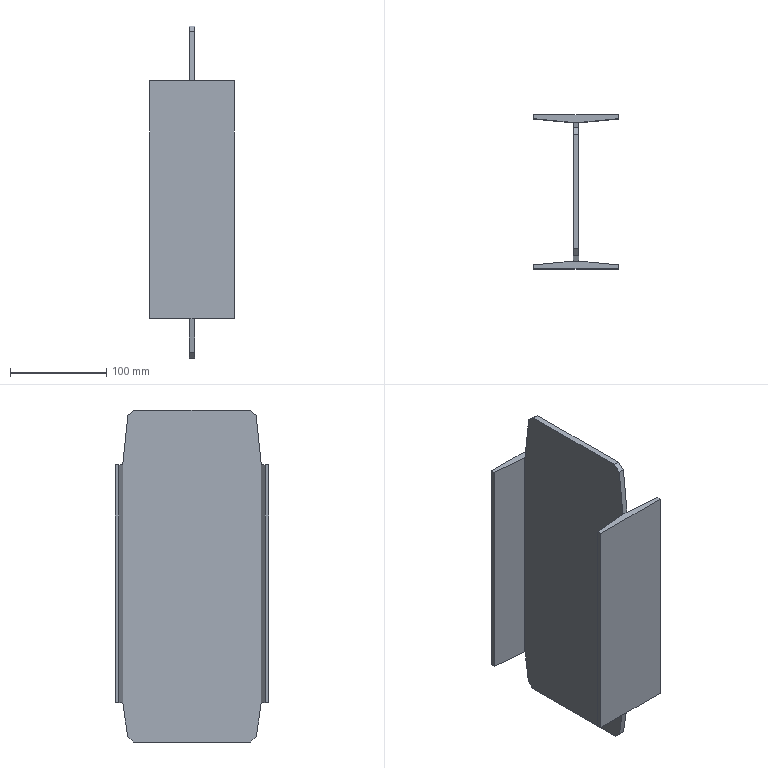Part | SolidWorks | features Chamfer 2, Extrusion 1, ICE 1 | 1 solid | 26 faces | box 88 x 160 x 345 mm | volume 560895 mm3 | plane 26
STEP:
#1=CARTESIAN_POINT('',(44.,-80.,115.5));
#2=VERTEX_POINT('',#1);
#3=CARTESIAN_POINT('',(44.,-80.,-131.5));
#4=VERTEX_POINT('',#3);
#5=CARTESIAN_POINT('',(44.,-80.,172.5));
#6=DIRECTION('',(0.,0.,-1.));
#7=VECTOR('',#6,1000.);
#8=LINE('',#5,#7);
#9=EDGE_CURVE('',#2,#4,#8,.T.);
#10=ORIENTED_EDGE('',*,*,#9,.F.);
#11=CARTESIAN_POINT('',(-44.,-80.,115.5));
#12=VERTEX_POINT('',#11);
#13=CARTESIAN_POINT('',(-44.,-80.,115.5));
#14=DIRECTION('',(1.,0.,0.));
#15=VECTOR('',#14,1000.);
#16=LINE('',#13,#15);
#17=EDGE_CURVE('',#12,#2,#16,.T.);
#18=ORIENTED_EDGE('',*,*,#17,.F.);
#19=CARTESIAN_POINT('',(-44.,-80.,-131.5));
#20=VERTEX_POINT('',#19);
#21=CARTESIAN_POINT('',(-44.,-80.,172.5));
#22=DIRECTION('',(0.,0.,-1.));
#23=VECTOR('',#22,1000.);
#24=LINE('',#21,#23);
#25=EDGE_CURVE('',#12,#20,#24,.T.);
#26=ORIENTED_EDGE('',*,*,#25,.T.);
#27=CARTESIAN_POINT('',(-44.,-80.,-131.5));
#28=DIRECTION('',(1.,0.,0.));
#29=VECTOR('',#28,1000.);
#30=LINE('',#27,#29);
#31=EDGE_CURVE('',#20,#4,#30,.T.);
#32=ORIENTED_EDGE('',*,*,#31,.T.);
#33=EDGE_LOOP('',(#10,#18,#26,#32));
#34=FACE_OUTER_BOUND('',#33,.T.);
#35=CARTESIAN_POINT('',(44.,-80.,172.5));
#36=DIRECTION('',(0.,1.,0.));
#37=DIRECTION('',(-1.,0.,0.));
#38=AXIS2_PLACEMENT_3D('',#35,#36,#37);
#39=PLANE('',#38);
#40=ADVANCED_FACE('',(#34),#39,.F.);
#41=CARTESIAN_POINT('',(44.,-76.,115.5));
#42=VERTEX_POINT('',#41);
#43=CARTESIAN_POINT('',(44.,-76.,-131.5));
#44=VERTEX_POINT('',#43);
#45=CARTESIAN_POINT('',(44.,-76.,172.5));
#46=DIRECTION('',(0.,0.,-1.));
#47=VECTOR('',#46,1000.);
#48=LINE('',#45,#47);
#49=EDGE_CURVE('',#42,#44,#48,.T.);
#50=ORIENTED_EDGE('',*,*,#49,.F.);
#51=CARTESIAN_POINT('',(44.,-72.,115.5));
#52=DIRECTION('',(0.,1.,0.));
#53=VECTOR('',#52,1000.);
#54=LINE('',#51,#53);
#55=EDGE_CURVE('',#2,#42,#54,.T.);
#56=ORIENTED_EDGE('',*,*,#55,.F.);
#57=ORIENTED_EDGE('',*,*,#9,.T.);
#58=CARTESIAN_POINT('',(44.,-72.,-131.5));
#59=DIRECTION('',(0.,-1.,0.));
#60=VECTOR('',#59,1000.);
#61=LINE('',#58,#60);
#62=EDGE_CURVE('',#44,#4,#61,.T.);
#63=ORIENTED_EDGE('',*,*,#62,.F.);
#64=EDGE_LOOP('',(#50,#56,#57,#63));
#65=FACE_OUTER_BOUND('',#64,.T.);
#66=CARTESIAN_POINT('',(44.,-80.,172.5));
#67=DIRECTION('',(-1.,0.,0.));
#68=DIRECTION('',(0.,-1.,0.));
#69=AXIS2_PLACEMENT_3D('',#66,#67,#68);
#70=PLANE('',#69);
#71=ADVANCED_FACE('',(#65),#70,.F.);
#72=CARTESIAN_POINT('',(3.,-72.,115.5));
#73=VERTEX_POINT('',#72);
#74=CARTESIAN_POINT('',(3.,-72.,-131.5));
#75=VERTEX_POINT('',#74);
#76=CARTESIAN_POINT('',(3.,-72.,172.5));
#77=DIRECTION('',(0.,0.,-1.));
#78=VECTOR('',#77,1000.);
#79=LINE('',#76,#78);
#80=EDGE_CURVE('',#73,#75,#79,.T.);
#81=ORIENTED_EDGE('',*,*,#80,.F.);
#82=CARTESIAN_POINT('',(44.,-76.,115.5));
#83=DIRECTION('',(0.9953,-0.0971,0.));
#84=VECTOR('',#83,1000.);
#85=LINE('',#82,#84);
#86=EDGE_CURVE('',#73,#42,#85,.T.);
#87=ORIENTED_EDGE('',*,*,#86,.T.);
#88=ORIENTED_EDGE('',*,*,#49,.T.);
#89=CARTESIAN_POINT('',(44.,-76.,-131.5));
#90=DIRECTION('',(-0.9953,0.0971,0.));
#91=VECTOR('',#90,1000.);
#92=LINE('',#89,#91);
#93=EDGE_CURVE('',#44,#75,#92,.T.);
#94=ORIENTED_EDGE('',*,*,#93,.T.);
#95=EDGE_LOOP('',(#81,#87,#88,#94));
#96=FACE_OUTER_BOUND('',#95,.T.);
#97=CARTESIAN_POINT('',(44.,-76.,172.5));
#98=DIRECTION('',(-0.0971,-0.9953,0.));
#99=DIRECTION('',(0.9953,-0.0971,0.));
#100=AXIS2_PLACEMENT_3D('',#97,#98,#99);
#101=PLANE('',#100);
#102=ADVANCED_FACE('',(#96),#101,.F.);
#103=CARTESIAN_POINT('',(3.,-66.857,-166.643));
#104=VERTEX_POINT('',#103);
#105=CARTESIAN_POINT('',(3.,-112.536,145.495));
#106=DIRECTION('',(0.,0.1448,-0.9895));
#107=VECTOR('',#106,1000.);
#108=LINE('',#105,#107);
#109=EDGE_CURVE('',#75,#104,#108,.T.);
#110=ORIENTED_EDGE('',*,*,#109,.T.);
#111=CARTESIAN_POINT('',(3.,-61.,-172.5));
#112=VERTEX_POINT('',#111);
#113=CARTESIAN_POINT('',(3.,-66.857,-166.643));
#114=DIRECTION('',(0.,0.7071,-0.7071));
#115=VECTOR('',#114,1000.);
#116=LINE('',#113,#115);
#117=EDGE_CURVE('',#104,#112,#116,.T.);
#118=ORIENTED_EDGE('',*,*,#117,.T.);
#119=CARTESIAN_POINT('',(3.,61.,-172.5));
#120=VERTEX_POINT('',#119);
#121=CARTESIAN_POINT('',(3.,72.,-172.5));
#122=DIRECTION('',(0.,1.,0.));
#123=VECTOR('',#122,1000.);
#124=LINE('',#121,#123);
#125=EDGE_CURVE('',#112,#120,#124,.T.);
#126=ORIENTED_EDGE('',*,*,#125,.T.);
#127=CARTESIAN_POINT('',(3.,66.857,-166.643));
#128=VERTEX_POINT('',#127);
#129=CARTESIAN_POINT('',(3.,66.857,-166.643));
#130=DIRECTION('',(0.,0.7071,0.7071));
#131=VECTOR('',#130,1000.);
#132=LINE('',#129,#131);
#133=EDGE_CURVE('',#120,#128,#132,.T.);
#134=ORIENTED_EDGE('',*,*,#133,.T.);
#135=CARTESIAN_POINT('',(3.,72.,-131.5));
#136=VERTEX_POINT('',#135);
#137=CARTESIAN_POINT('',(3.,115.555,166.126));
#138=DIRECTION('',(0.,0.1448,0.9895));
#139=VECTOR('',#138,1000.);
#140=LINE('',#137,#139);
#141=EDGE_CURVE('',#128,#136,#140,.T.);
#142=ORIENTED_EDGE('',*,*,#141,.T.);
#143=CARTESIAN_POINT('',(3.,72.,115.5));
#144=VERTEX_POINT('',#143);
#145=CARTESIAN_POINT('',(3.,72.,172.5));
#146=DIRECTION('',(0.,0.,-1.));
#147=VECTOR('',#146,1000.);
#148=LINE('',#145,#147);
#149=EDGE_CURVE('',#144,#136,#148,.T.);
#150=ORIENTED_EDGE('',*,*,#149,.F.);
#151=CARTESIAN_POINT('',(3.,66.628,166.533));
#152=VERTEX_POINT('',#151);
#153=CARTESIAN_POINT('',(3.,66.066,171.875));
#154=DIRECTION('',(0.,-0.1047,0.9945));
#155=VECTOR('',#154,1000.);
#156=LINE('',#153,#155);
#157=EDGE_CURVE('',#144,#152,#156,.T.);
#158=ORIENTED_EDGE('',*,*,#157,.T.);
#159=CARTESIAN_POINT('',(3.,59.257,172.5));
#160=VERTEX_POINT('',#159);
#161=CARTESIAN_POINT('',(3.,59.257,172.5));
#162=DIRECTION('',(0.,-0.7772,0.6292));
#163=VECTOR('',#162,1000.);
#164=LINE('',#161,#163);
#165=EDGE_CURVE('',#152,#160,#164,.T.);
#166=ORIENTED_EDGE('',*,*,#165,.T.);
#167=CARTESIAN_POINT('',(3.,-59.257,172.5));
#168=VERTEX_POINT('',#167);
#169=CARTESIAN_POINT('',(3.,72.,172.5));
#170=DIRECTION('',(0.,1.,0.));
#171=VECTOR('',#170,1000.);
#172=LINE('',#169,#171);
#173=EDGE_CURVE('',#168,#160,#172,.T.);
#174=ORIENTED_EDGE('',*,*,#173,.F.);
#175=CARTESIAN_POINT('',(3.,-66.628,166.533));
#176=VERTEX_POINT('',#175);
#177=CARTESIAN_POINT('',(3.,-59.257,172.5));
#178=DIRECTION('',(0.,-0.7772,-0.6292));
#179=VECTOR('',#178,1000.);
#180=LINE('',#177,#179);
#181=EDGE_CURVE('',#168,#176,#180,.T.);
#182=ORIENTED_EDGE('',*,*,#181,.T.);
#183=CARTESIAN_POINT('',(3.,-64.488,186.867));
#184=DIRECTION('',(0.,-0.1047,-0.9945));
#185=VECTOR('',#184,1000.);
#186=LINE('',#183,#185);
#187=EDGE_CURVE('',#176,#73,#186,.T.);
#188=ORIENTED_EDGE('',*,*,#187,.T.);
#189=ORIENTED_EDGE('',*,*,#80,.T.);
#190=EDGE_LOOP('',(#110,#118,#126,#134,#142,#150,#158,#166,#174,#182,#188,#189));
#191=FACE_OUTER_BOUND('',#190,.T.);
#192=CARTESIAN_POINT('',(3.,72.,172.5));
#193=DIRECTION('',(-1.,0.,0.));
#194=DIRECTION('',(0.,0.,1.));
#195=AXIS2_PLACEMENT_3D('',#192,#193,#194);
#196=PLANE('',#195);
#197=ADVANCED_FACE('',(#191),#196,.F.);
#198=ORIENTED_EDGE('',*,*,#149,.T.);
#199=CARTESIAN_POINT('',(44.,76.,-131.5));
#200=VERTEX_POINT('',#199);
#201=CARTESIAN_POINT('',(44.,76.,-131.5));
#202=DIRECTION('',(0.9953,0.0971,0.));
#203=VECTOR('',#202,1000.);
#204=LINE('',#201,#203);
#205=EDGE_CURVE('',#136,#200,#204,.T.);
#206=ORIENTED_EDGE('',*,*,#205,.T.);
#207=CARTESIAN_POINT('',(44.,76.,115.5));
#208=VERTEX_POINT('',#207);
#209=CARTESIAN_POINT('',(44.,76.,172.5));
#210=DIRECTION('',(0.,0.,-1.));
#211=VECTOR('',#210,1000.);
#212=LINE('',#209,#211);
#213=EDGE_CURVE('',#208,#200,#212,.T.);
#214=ORIENTED_EDGE('',*,*,#213,.F.);
#215=CARTESIAN_POINT('',(44.,76.,115.5));
#216=DIRECTION('',(-0.9953,-0.0971,0.));
#217=VECTOR('',#216,1000.);
#218=LINE('',#215,#217);
#219=EDGE_CURVE('',#208,#144,#218,.T.);
#220=ORIENTED_EDGE('',*,*,#219,.T.);
#221=EDGE_LOOP('',(#198,#206,#214,#220));
#222=FACE_OUTER_BOUND('',#221,.T.);
#223=CARTESIAN_POINT('',(44.,76.,172.5));
#224=DIRECTION('',(-0.0971,0.9953,0.));
#225=DIRECTION('',(-0.9953,-0.0971,0.));
#226=AXIS2_PLACEMENT_3D('',#223,#224,#225);
#227=PLANE('',#226);
#228=ADVANCED_FACE('',(#222),#227,.F.);
#229=ORIENTED_EDGE('',*,*,#213,.T.);
#230=CARTESIAN_POINT('',(44.,80.,-131.5));
#231=VERTEX_POINT('',#230);
#232=CARTESIAN_POINT('',(44.,72.,-131.5));
#233=DIRECTION('',(0.,-1.,0.));
#234=VECTOR('',#233,1000.);
#235=LINE('',#232,#234);
#236=EDGE_CURVE('',#231,#200,#235,.T.);
#237=ORIENTED_EDGE('',*,*,#236,.F.);
#238=CARTESIAN_POINT('',(44.,80.,115.5));
#239=VERTEX_POINT('',#238);
#240=CARTESIAN_POINT('',(44.,80.,172.5));
#241=DIRECTION('',(0.,0.,-1.));
#242=VECTOR('',#241,1000.);
#243=LINE('',#240,#242);
#244=EDGE_CURVE('',#239,#231,#243,.T.);
#245=ORIENTED_EDGE('',*,*,#244,.F.);
#246=CARTESIAN_POINT('',(44.,72.,115.5));
#247=DIRECTION('',(0.,1.,0.));
#248=VECTOR('',#247,1000.);
#249=LINE('',#246,#248);
#250=EDGE_CURVE('',#208,#239,#249,.T.);
#251=ORIENTED_EDGE('',*,*,#250,.F.);
#252=EDGE_LOOP('',(#229,#237,#245,#251));
#253=FACE_OUTER_BOUND('',#252,.T.);
#254=CARTESIAN_POINT('',(44.,80.,172.5));
#255=DIRECTION('',(-1.,0.,0.));
#256=DIRECTION('',(0.,0.,1.));
#257=AXIS2_PLACEMENT_3D('',#254,#255,#256);
#258=PLANE('',#257);
#259=ADVANCED_FACE('',(#253),#258,.F.);
#260=ORIENTED_EDGE('',*,*,#244,.T.);
#261=CARTESIAN_POINT('',(-44.,80.,-131.5));
#262=VERTEX_POINT('',#261);
#263=CARTESIAN_POINT('',(-44.,80.,-131.5));
#264=DIRECTION('',(1.,0.,0.));
#265=VECTOR('',#264,1000.);
#266=LINE('',#263,#265);
#267=EDGE_CURVE('',#262,#231,#266,.T.);
#268=ORIENTED_EDGE('',*,*,#267,.F.);
#269=CARTESIAN_POINT('',(-44.,80.,115.5));
#270=VERTEX_POINT('',#269);
#271=CARTESIAN_POINT('',(-44.,80.,172.5));
#272=DIRECTION('',(0.,0.,-1.));
#273=VECTOR('',#272,1000.);
#274=LINE('',#271,#273);
#275=EDGE_CURVE('',#270,#262,#274,.T.);
#276=ORIENTED_EDGE('',*,*,#275,.F.);
#277=CARTESIAN_POINT('',(-44.,80.,115.5));
#278=DIRECTION('',(1.,0.,0.));
#279=VECTOR('',#278,1000.);
#280=LINE('',#277,#279);
#281=EDGE_CURVE('',#270,#239,#280,.T.);
#282=ORIENTED_EDGE('',*,*,#281,.T.);
#283=EDGE_LOOP('',(#260,#268,#276,#282));
#284=FACE_OUTER_BOUND('',#283,.T.);
#285=CARTESIAN_POINT('',(44.,80.,172.5));
#286=DIRECTION('',(0.,-1.,0.));
#287=DIRECTION('',(1.,0.,0.));
#288=AXIS2_PLACEMENT_3D('',#285,#286,#287);
#289=PLANE('',#288);
#290=ADVANCED_FACE('',(#284),#289,.F.);
#291=ORIENTED_EDGE('',*,*,#275,.T.);
#292=CARTESIAN_POINT('',(-44.,76.,-131.5));
#293=VERTEX_POINT('',#292);
#294=CARTESIAN_POINT('',(-44.,72.,-131.5));
#295=DIRECTION('',(0.,-1.,0.));
#296=VECTOR('',#295,1000.);
#297=LINE('',#294,#296);
#298=EDGE_CURVE('',#262,#293,#297,.T.);
#299=ORIENTED_EDGE('',*,*,#298,.T.);
#300=CARTESIAN_POINT('',(-44.,76.,115.5));
#301=VERTEX_POINT('',#300);
#302=CARTESIAN_POINT('',(-44.,76.,172.5));
#303=DIRECTION('',(0.,0.,-1.));
#304=VECTOR('',#303,1000.);
#305=LINE('',#302,#304);
#306=EDGE_CURVE('',#301,#293,#305,.T.);
#307=ORIENTED_EDGE('',*,*,#306,.F.);
#308=CARTESIAN_POINT('',(-44.,72.,115.5));
#309=DIRECTION('',(0.,1.,0.));
#310=VECTOR('',#309,1000.);
#311=LINE('',#308,#310);
#312=EDGE_CURVE('',#301,#270,#311,.T.);
#313=ORIENTED_EDGE('',*,*,#312,.T.);
#314=EDGE_LOOP('',(#291,#299,#307,#313));
#315=FACE_OUTER_BOUND('',#314,.T.);
#316=CARTESIAN_POINT('',(-44.,80.,172.5));
#317=DIRECTION('',(1.,0.,0.));
#318=DIRECTION('',(0.,1.,0.));
#319=AXIS2_PLACEMENT_3D('',#316,#317,#318);
#320=PLANE('',#319);
#321=ADVANCED_FACE('',(#315),#320,.F.);
#322=ORIENTED_EDGE('',*,*,#306,.T.);
#323=CARTESIAN_POINT('',(-3.,72.,-131.5));
#324=VERTEX_POINT('',#323);
#325=CARTESIAN_POINT('',(-44.,76.,-131.5));
#326=DIRECTION('',(0.9953,-0.0971,0.));
#327=VECTOR('',#326,1000.);
#328=LINE('',#325,#327);
#329=EDGE_CURVE('',#293,#324,#328,.T.);
#330=ORIENTED_EDGE('',*,*,#329,.T.);
#331=CARTESIAN_POINT('',(-3.,72.,115.5));
#332=VERTEX_POINT('',#331);
#333=CARTESIAN_POINT('',(-3.,72.,172.5));
#334=DIRECTION('',(0.,0.,-1.));
#335=VECTOR('',#334,1000.);
#336=LINE('',#333,#335);
#337=EDGE_CURVE('',#332,#324,#336,.T.);
#338=ORIENTED_EDGE('',*,*,#337,.F.);
#339=CARTESIAN_POINT('',(-44.,76.,115.5));
#340=DIRECTION('',(-0.9953,0.0971,0.));
#341=VECTOR('',#340,1000.);
#342=LINE('',#339,#341);
#343=EDGE_CURVE('',#332,#301,#342,.T.);
#344=ORIENTED_EDGE('',*,*,#343,.T.);
#345=EDGE_LOOP('',(#322,#330,#338,#344));
#346=FACE_OUTER_BOUND('',#345,.T.);
#347=CARTESIAN_POINT('',(-44.,76.,172.5));
#348=DIRECTION('',(0.0971,0.9953,0.));
#349=DIRECTION('',(-0.9953,0.0971,0.));
#350=AXIS2_PLACEMENT_3D('',#347,#348,#349);
#351=PLANE('',#350);
#352=ADVANCED_FACE('',(#346),#351,.F.);
#353=CARTESIAN_POINT('',(-3.,61.,-172.5));
#354=VERTEX_POINT('',#353);
#355=CARTESIAN_POINT('',(-3.,-61.,-172.5));
#356=VERTEX_POINT('',#355);
#357=CARTESIAN_POINT('',(-3.,72.,-172.5));
#358=DIRECTION('',(0.,-1.,0.));
#359=VECTOR('',#358,1000.);
#360=LINE('',#357,#359);
#361=EDGE_CURVE('',#354,#356,#360,.T.);
#362=ORIENTED_EDGE('',*,*,#361,.T.);
#363=CARTESIAN_POINT('',(-3.,-66.857,-166.643));
#364=VERTEX_POINT('',#363);
#365=CARTESIAN_POINT('',(-3.,-66.857,-166.643));
#366=DIRECTION('',(0.,-0.7071,0.7071));
#367=VECTOR('',#366,1000.);
#368=LINE('',#365,#367);
#369=EDGE_CURVE('',#356,#364,#368,.T.);
#370=ORIENTED_EDGE('',*,*,#369,.T.);
#371=CARTESIAN_POINT('',(-3.,-72.,-131.5));
#372=VERTEX_POINT('',#371);
#373=CARTESIAN_POINT('',(-3.,-112.536,145.495));
#374=DIRECTION('',(0.,-0.1448,0.9895));
#375=VECTOR('',#374,1000.);
#376=LINE('',#373,#375);
#377=EDGE_CURVE('',#364,#372,#376,.T.);
#378=ORIENTED_EDGE('',*,*,#377,.T.);
#379=CARTESIAN_POINT('',(-3.,-72.,115.5));
#380=VERTEX_POINT('',#379);
#381=CARTESIAN_POINT('',(-3.,-72.,172.5));
#382=DIRECTION('',(0.,0.,-1.));
#383=VECTOR('',#382,1000.);
#384=LINE('',#381,#383);
#385=EDGE_CURVE('',#380,#372,#384,.T.);
#386=ORIENTED_EDGE('',*,*,#385,.F.);
#387=CARTESIAN_POINT('',(-3.,-66.628,166.533));
#388=VERTEX_POINT('',#387);
#389=CARTESIAN_POINT('',(-3.,-64.488,186.867));
#390=DIRECTION('',(0.,0.1047,0.9945));
#391=VECTOR('',#390,1000.);
#392=LINE('',#389,#391);
#393=EDGE_CURVE('',#380,#388,#392,.T.);
#394=ORIENTED_EDGE('',*,*,#393,.T.);
#395=CARTESIAN_POINT('',(-3.,-59.257,172.5));
#396=VERTEX_POINT('',#395);
#397=CARTESIAN_POINT('',(-3.,-59.257,172.5));
#398=DIRECTION('',(0.,0.7772,0.6292));
#399=VECTOR('',#398,1000.);
#400=LINE('',#397,#399);
#401=EDGE_CURVE('',#388,#396,#400,.T.);
#402=ORIENTED_EDGE('',*,*,#401,.T.);
#403=CARTESIAN_POINT('',(-3.,59.257,172.5));
#404=VERTEX_POINT('',#403);
#405=CARTESIAN_POINT('',(-3.,72.,172.5));
#406=DIRECTION('',(0.,-1.,0.));
#407=VECTOR('',#406,1000.);
#408=LINE('',#405,#407);
#409=EDGE_CURVE('',#404,#396,#408,.T.);
#410=ORIENTED_EDGE('',*,*,#409,.F.);
#411=CARTESIAN_POINT('',(-3.,66.628,166.533));
#412=VERTEX_POINT('',#411);
#413=CARTESIAN_POINT('',(-3.,59.257,172.5));
#414=DIRECTION('',(0.,0.7772,-0.6292));
#415=VECTOR('',#414,1000.);
#416=LINE('',#413,#415);
#417=EDGE_CURVE('',#404,#412,#416,.T.);
#418=ORIENTED_EDGE('',*,*,#417,.T.);
#419=CARTESIAN_POINT('',(-3.,66.066,171.875));
#420=DIRECTION('',(0.,0.1047,-0.9945));
#421=VECTOR('',#420,1000.);
#422=LINE('',#419,#421);
#423=EDGE_CURVE('',#412,#332,#422,.T.);
#424=ORIENTED_EDGE('',*,*,#423,.T.);
#425=ORIENTED_EDGE('',*,*,#337,.T.);
#426=CARTESIAN_POINT('',(-3.,66.857,-166.643));
#427=VERTEX_POINT('',#426);
#428=CARTESIAN_POINT('',(-3.,115.555,166.126));
#429=DIRECTION('',(0.,-0.1448,-0.9895));
#430=VECTOR('',#429,1000.);
#431=LINE('',#428,#430);
#432=EDGE_CURVE('',#324,#427,#431,.T.);
#433=ORIENTED_EDGE('',*,*,#432,.T.);
#434=CARTESIAN_POINT('',(-3.,66.857,-166.643));
#435=DIRECTION('',(0.,-0.7071,-0.7071));
#436=VECTOR('',#435,1000.);
#437=LINE('',#434,#436);
#438=EDGE_CURVE('',#427,#354,#437,.T.);
#439=ORIENTED_EDGE('',*,*,#438,.T.);
#440=EDGE_LOOP('',(#362,#370,#378,#386,#394,#402,#410,#418,#424,#425,#433,#439));
#441=FACE_OUTER_BOUND('',#440,.T.);
#442=CARTESIAN_POINT('',(-3.,72.,172.5));
#443=DIRECTION('',(1.,0.,0.));
#444=DIRECTION('',(0.,0.,-1.));
#445=AXIS2_PLACEMENT_3D('',#442,#443,#444);
#446=PLANE('',#445);
#447=ADVANCED_FACE('',(#441),#446,.F.);
#448=CARTESIAN_POINT('',(-44.,-76.,115.5));
#449=VERTEX_POINT('',#448);
#450=CARTESIAN_POINT('',(-44.,-76.,-131.5));
#451=VERTEX_POINT('',#450);
#452=CARTESIAN_POINT('',(-44.,-76.,172.5));
#453=DIRECTION('',(0.,0.,-1.));
#454=VECTOR('',#453,1000.);
#455=LINE('',#452,#454);
#456=EDGE_CURVE('',#449,#451,#455,.T.);
#457=ORIENTED_EDGE('',*,*,#456,.F.);
#458=CARTESIAN_POINT('',(-44.,-76.,115.5));
#459=DIRECTION('',(0.9953,0.0971,0.));
#460=VECTOR('',#459,1000.);
#461=LINE('',#458,#460);
#462=EDGE_CURVE('',#449,#380,#461,.T.);
#463=ORIENTED_EDGE('',*,*,#462,.T.);
#464=ORIENTED_EDGE('',*,*,#385,.T.);
#465=CARTESIAN_POINT('',(-44.,-76.,-131.5));
#466=DIRECTION('',(-0.9953,-0.0971,0.));
#467=VECTOR('',#466,1000.);
#468=LINE('',#465,#467);
#469=EDGE_CURVE('',#372,#451,#468,.T.);
#470=ORIENTED_EDGE('',*,*,#469,.T.);
#471=EDGE_LOOP('',(#457,#463,#464,#470));
#472=FACE_OUTER_BOUND('',#471,.T.);
#473=CARTESIAN_POINT('',(-44.,-76.,172.5));
#474=DIRECTION('',(0.0971,-0.9953,0.));
#475=DIRECTION('',(0.9953,0.0971,0.));
#476=AXIS2_PLACEMENT_3D('',#473,#474,#475);
#477=PLANE('',#476);
#478=ADVANCED_FACE('',(#472),#477,.F.);
#479=ORIENTED_EDGE('',*,*,#25,.F.);
#480=CARTESIAN_POINT('',(-44.,-72.,115.5));
#481=DIRECTION('',(0.,1.,0.));
#482=VECTOR('',#481,1000.);
#483=LINE('',#480,#482);
#484=EDGE_CURVE('',#12,#449,#483,.T.);
#485=ORIENTED_EDGE('',*,*,#484,.T.);
#486=ORIENTED_EDGE('',*,*,#456,.T.);
#487=CARTESIAN_POINT('',(-44.,-72.,-131.5));
#488=DIRECTION('',(0.,-1.,0.));
#489=VECTOR('',#488,1000.);
#490=LINE('',#487,#489);
#491=EDGE_CURVE('',#451,#20,#490,.T.);
#492=ORIENTED_EDGE('',*,*,#491,.T.);
#493=EDGE_LOOP('',(#479,#485,#486,#492));
#494=FACE_OUTER_BOUND('',#493,.T.);
#495=CARTESIAN_POINT('',(-44.,-80.,172.5));
#496=DIRECTION('',(1.,0.,0.));
#497=DIRECTION('',(0.,1.,0.));
#498=AXIS2_PLACEMENT_3D('',#495,#496,#497);
#499=PLANE('',#498);
#500=ADVANCED_FACE('',(#494),#499,.F.);
#501=ORIENTED_EDGE('',*,*,#409,.T.);
#502=CARTESIAN_POINT('',(0.,-59.257,172.5));
#503=DIRECTION('',(1.,0.,0.));
#504=VECTOR('',#503,1000.);
#505=LINE('',#502,#504);
#506=EDGE_CURVE('',#396,#168,#505,.T.);
#507=ORIENTED_EDGE('',*,*,#506,.T.);
#508=ORIENTED_EDGE('',*,*,#173,.T.);
#509=CARTESIAN_POINT('',(0.,59.257,172.5));
#510=DIRECTION('',(-1.,0.,0.));
#511=VECTOR('',#510,1000.);
#512=LINE('',#509,#511);
#513=EDGE_CURVE('',#160,#404,#512,.T.);
#514=ORIENTED_EDGE('',*,*,#513,.T.);
#515=EDGE_LOOP('',(#501,#507,#508,#514));
#516=FACE_OUTER_BOUND('',#515,.T.);
#517=CARTESIAN_POINT('',(0.,0.,172.5));
#518=DIRECTION('',(0.,0.,-1.));
#519=DIRECTION('',(-1.,0.,0.));
#520=AXIS2_PLACEMENT_3D('',#517,#518,#519);
#521=PLANE('',#520);
#522=ADVANCED_FACE('',(#516),#521,.F.);
#523=ORIENTED_EDGE('',*,*,#125,.F.);
#524=CARTESIAN_POINT('',(-3.,-61.,-172.5));
#525=DIRECTION('',(-1.,0.,0.));
#526=VECTOR('',#525,1000.);
#527=LINE('',#524,#526);
#528=EDGE_CURVE('',#112,#356,#527,.T.);
#529=ORIENTED_EDGE('',*,*,#528,.T.);
#530=ORIENTED_EDGE('',*,*,#361,.F.);
#531=CARTESIAN_POINT('',(3.,61.,-172.5));
#532=DIRECTION('',(1.,0.,0.));
#533=VECTOR('',#532,1000.);
#534=LINE('',#531,#533);
#535=EDGE_CURVE('',#354,#120,#534,.T.);
#536=ORIENTED_EDGE('',*,*,#535,.T.);
#537=EDGE_LOOP('',(#523,#529,#530,#536));
#538=FACE_OUTER_BOUND('',#537,.T.);
#539=CARTESIAN_POINT('',(0.,0.,-172.5));
#540=DIRECTION('',(0.,0.,-1.));
#541=DIRECTION('',(-1.,0.,0.));
#542=AXIS2_PLACEMENT_3D('',#539,#540,#541);
#543=PLANE('',#542);
#544=ADVANCED_FACE('',(#538),#543,.T.);
#545=CARTESIAN_POINT('',(-44.,72.,-131.5));
#546=DIRECTION('',(1.,0.,0.));
#547=VECTOR('',#546,1000.);
#548=LINE('',#545,#547);
#549=EDGE_CURVE('',#324,#136,#548,.T.);
#550=ORIENTED_EDGE('',*,*,#549,.F.);
#551=ORIENTED_EDGE('',*,*,#329,.F.);
#552=ORIENTED_EDGE('',*,*,#298,.F.);
#553=ORIENTED_EDGE('',*,*,#267,.T.);
#554=ORIENTED_EDGE('',*,*,#236,.T.);
#555=ORIENTED_EDGE('',*,*,#205,.F.);
#556=EDGE_LOOP('',(#550,#551,#552,#553,#554,#555));
#557=FACE_OUTER_BOUND('',#556,.T.);
#558=CARTESIAN_POINT('',(-44.,72.,-131.5));
#559=DIRECTION('',(0.,0.,1.));
#560=DIRECTION('',(0.,-1.,0.));
#561=AXIS2_PLACEMENT_3D('',#558,#559,#560);
#562=PLANE('',#561);
#563=ADVANCED_FACE('',(#557),#562,.F.);
#564=ORIENTED_EDGE('',*,*,#141,.F.);
#565=CARTESIAN_POINT('',(-3.,66.857,-166.643));
#566=DIRECTION('',(-1.,0.,0.));
#567=VECTOR('',#566,1000.);
#568=LINE('',#565,#567);
#569=EDGE_CURVE('',#128,#427,#568,.T.);
#570=ORIENTED_EDGE('',*,*,#569,.T.);
#571=ORIENTED_EDGE('',*,*,#432,.F.);
#572=ORIENTED_EDGE('',*,*,#549,.T.);
#573=EDGE_LOOP('',(#564,#570,#571,#572));
#574=FACE_OUTER_BOUND('',#573,.T.);
#575=CARTESIAN_POINT('',(-44.,66.,-172.5));
#576=DIRECTION('',(0.,-0.9895,0.1448));
#577=DIRECTION('',(0.,-0.1448,-0.9895));
#578=AXIS2_PLACEMENT_3D('',#575,#576,#577);
#579=PLANE('',#578);
#580=ADVANCED_FACE('',(#574),#579,.F.);
#581=ORIENTED_EDGE('',*,*,#62,.T.);
#582=ORIENTED_EDGE('',*,*,#31,.F.);
#583=ORIENTED_EDGE('',*,*,#491,.F.);
#584=ORIENTED_EDGE('',*,*,#469,.F.);
#585=CARTESIAN_POINT('',(-44.,-72.,-131.5));
#586=DIRECTION('',(1.,0.,0.));
#587=VECTOR('',#586,1000.);
#588=LINE('',#585,#587);
#589=EDGE_CURVE('',#372,#75,#588,.T.);
#590=ORIENTED_EDGE('',*,*,#589,.T.);
#591=ORIENTED_EDGE('',*,*,#93,.F.);
#592=EDGE_LOOP('',(#581,#582,#583,#584,#590,#591));
#593=FACE_OUTER_BOUND('',#592,.T.);
#594=CARTESIAN_POINT('',(-44.,-72.,-131.5));
#595=DIRECTION('',(0.,0.,1.));
#596=DIRECTION('',(0.,-1.,0.));
#597=AXIS2_PLACEMENT_3D('',#594,#595,#596);
#598=PLANE('',#597);
#599=ADVANCED_FACE('',(#593),#598,.F.);
#600=ORIENTED_EDGE('',*,*,#377,.F.);
#601=CARTESIAN_POINT('',(3.,-66.857,-166.643));
#602=DIRECTION('',(1.,0.,0.));
#603=VECTOR('',#602,1000.);
#604=LINE('',#601,#603);
#605=EDGE_CURVE('',#364,#104,#604,.T.);
#606=ORIENTED_EDGE('',*,*,#605,.T.);
#607=ORIENTED_EDGE('',*,*,#109,.F.);
#608=ORIENTED_EDGE('',*,*,#589,.F.);
#609=EDGE_LOOP('',(#600,#606,#607,#608));
#610=FACE_OUTER_BOUND('',#609,.T.);
#611=CARTESIAN_POINT('',(-44.,-66.,-172.5));
#612=DIRECTION('',(0.,0.9895,0.1448));
#613=DIRECTION('',(0.,-0.1448,0.9895));
#614=AXIS2_PLACEMENT_3D('',#611,#612,#613);
#615=PLANE('',#614);
#616=ADVANCED_FACE('',(#610),#615,.F.);
#617=ORIENTED_EDGE('',*,*,#250,.T.);
#618=ORIENTED_EDGE('',*,*,#281,.F.);
#619=ORIENTED_EDGE('',*,*,#312,.F.);
#620=ORIENTED_EDGE('',*,*,#343,.F.);
#621=CARTESIAN_POINT('',(-44.,72.,115.5));
#622=DIRECTION('',(1.,0.,0.));
#623=VECTOR('',#622,1000.);
#624=LINE('',#621,#623);
#625=EDGE_CURVE('',#332,#144,#624,.T.);
#626=ORIENTED_EDGE('',*,*,#625,.T.);
#627=ORIENTED_EDGE('',*,*,#219,.F.);
#628=EDGE_LOOP('',(#617,#618,#619,#620,#626,#627));
#629=FACE_OUTER_BOUND('',#628,.T.);
#630=CARTESIAN_POINT('',(-44.,72.,115.5));
#631=DIRECTION('',(0.,0.,-1.));
#632=DIRECTION('',(-1.,0.,0.));
#633=AXIS2_PLACEMENT_3D('',#630,#631,#632);
#634=PLANE('',#633);
#635=ADVANCED_FACE('',(#629),#634,.F.);
#636=ORIENTED_EDGE('',*,*,#423,.F.);
#637=CARTESIAN_POINT('',(-44.,66.628,166.533));
#638=DIRECTION('',(1.,0.,0.));
#639=VECTOR('',#638,1000.);
#640=LINE('',#637,#639);
#641=EDGE_CURVE('',#412,#152,#640,.T.);
#642=ORIENTED_EDGE('',*,*,#641,.T.);
#643=ORIENTED_EDGE('',*,*,#157,.F.);
#644=ORIENTED_EDGE('',*,*,#625,.F.);
#645=EDGE_LOOP('',(#636,#642,#643,#644));
#646=FACE_OUTER_BOUND('',#645,.T.);
#647=CARTESIAN_POINT('',(-44.,66.,172.5));
#648=DIRECTION('',(0.,-0.9945,-0.1047));
#649=DIRECTION('',(0.,0.1047,-0.9945));
#650=AXIS2_PLACEMENT_3D('',#647,#648,#649);
#651=PLANE('',#650);
#652=ADVANCED_FACE('',(#646),#651,.F.);
#653=CARTESIAN_POINT('',(-44.,-72.,115.5));
#654=DIRECTION('',(1.,0.,0.));
#655=VECTOR('',#654,1000.);
#656=LINE('',#653,#655);
#657=EDGE_CURVE('',#380,#73,#656,.T.);
#658=ORIENTED_EDGE('',*,*,#657,.F.);
#659=ORIENTED_EDGE('',*,*,#462,.F.);
#660=ORIENTED_EDGE('',*,*,#484,.F.);
#661=ORIENTED_EDGE('',*,*,#17,.T.);
#662=ORIENTED_EDGE('',*,*,#55,.T.);
#663=ORIENTED_EDGE('',*,*,#86,.F.);
#664=EDGE_LOOP('',(#658,#659,#660,#661,#662,#663));
#665=FACE_OUTER_BOUND('',#664,.T.);
#666=CARTESIAN_POINT('',(-44.,-72.,115.5));
#667=DIRECTION('',(0.,0.,-1.));
#668=DIRECTION('',(-1.,0.,0.));
#669=AXIS2_PLACEMENT_3D('',#666,#667,#668);
#670=PLANE('',#669);
#671=ADVANCED_FACE('',(#665),#670,.F.);
#672=ORIENTED_EDGE('',*,*,#187,.F.);
#673=CARTESIAN_POINT('',(-44.,-66.628,166.533));
#674=DIRECTION('',(-1.,0.,0.));
#675=VECTOR('',#674,1000.);
#676=LINE('',#673,#675);
#677=EDGE_CURVE('',#176,#388,#676,.T.);
#678=ORIENTED_EDGE('',*,*,#677,.T.);
#679=ORIENTED_EDGE('',*,*,#393,.F.);
#680=ORIENTED_EDGE('',*,*,#657,.T.);
#681=EDGE_LOOP('',(#672,#678,#679,#680));
#682=FACE_OUTER_BOUND('',#681,.T.);
#683=CARTESIAN_POINT('',(-44.,-66.,172.5));
#684=DIRECTION('',(0.,0.9945,-0.1047));
#685=DIRECTION('',(0.,0.1047,0.9945));
#686=AXIS2_PLACEMENT_3D('',#683,#684,#685);
#687=PLANE('',#686);
#688=ADVANCED_FACE('',(#682),#687,.F.);
#689=ORIENTED_EDGE('',*,*,#401,.F.);
#690=ORIENTED_EDGE('',*,*,#677,.F.);
#691=ORIENTED_EDGE('',*,*,#181,.F.);
#692=ORIENTED_EDGE('',*,*,#506,.F.);
#693=EDGE_LOOP('',(#689,#690,#691,#692));
#694=FACE_OUTER_BOUND('',#693,.T.);
#695=CARTESIAN_POINT('',(0.,-59.257,172.5));
#696=DIRECTION('',(0.,0.6292,-0.7772));
#697=DIRECTION('',(1.,0.,0.));
#698=AXIS2_PLACEMENT_3D('',#695,#696,#697);
#699=PLANE('',#698);
#700=ADVANCED_FACE('',(#694),#699,.F.);
#701=ORIENTED_EDGE('',*,*,#165,.F.);
#702=ORIENTED_EDGE('',*,*,#641,.F.);
#703=ORIENTED_EDGE('',*,*,#417,.F.);
#704=ORIENTED_EDGE('',*,*,#513,.F.);
#705=EDGE_LOOP('',(#701,#702,#703,#704));
#706=FACE_OUTER_BOUND('',#705,.T.);
#707=CARTESIAN_POINT('',(0.,59.257,172.5));
#708=DIRECTION('',(0.,-0.6292,-0.7772));
#709=DIRECTION('',(-1.,0.,0.));
#710=AXIS2_PLACEMENT_3D('',#707,#708,#709);
#711=PLANE('',#710);
#712=ADVANCED_FACE('',(#706),#711,.F.);
#713=ORIENTED_EDGE('',*,*,#369,.F.);
#714=ORIENTED_EDGE('',*,*,#528,.F.);
#715=ORIENTED_EDGE('',*,*,#117,.F.);
#716=ORIENTED_EDGE('',*,*,#605,.F.);
#717=EDGE_LOOP('',(#713,#714,#715,#716));
#718=FACE_OUTER_BOUND('',#717,.T.);
#719=CARTESIAN_POINT('',(-44.,-66.857,-166.643));
#720=DIRECTION('',(0.,-0.7071,-0.7071));
#721=DIRECTION('',(-1.,0.,0.));
#722=AXIS2_PLACEMENT_3D('',#719,#720,#721);
#723=PLANE('',#722);
#724=ADVANCED_FACE('',(#718),#723,.T.);
#725=ORIENTED_EDGE('',*,*,#133,.F.);
#726=ORIENTED_EDGE('',*,*,#535,.F.);
#727=ORIENTED_EDGE('',*,*,#438,.F.);
#728=ORIENTED_EDGE('',*,*,#569,.F.);
#729=EDGE_LOOP('',(#725,#726,#727,#728));
#730=FACE_OUTER_BOUND('',#729,.T.);
#731=CARTESIAN_POINT('',(-44.,66.857,-166.643));
#732=DIRECTION('',(0.,0.7071,-0.7071));
#733=DIRECTION('',(1.,0.,0.));
#734=AXIS2_PLACEMENT_3D('',#731,#732,#733);
#735=PLANE('',#734);
#736=ADVANCED_FACE('',(#730),#735,.T.);
#737=CLOSED_SHELL('',(#40,#71,#102,#197,#228,#259,#290,#321,#352,#447,#478,#500,#522,#544,#563,#580,#599,#616,#635,#652,#671,#688,#700,#712,#724,#736));
#738=MANIFOLD_SOLID_BREP('',#737);
#739=CARTESIAN_POINT('',(0.,0.,0.));
#740=DIRECTION('',(0.,0.,1.));
#741=DIRECTION('',(1.,0.,0.));
#742=AXIS2_PLACEMENT_3D('',#739,#740,#741);
#743=(LENGTH_UNIT()NAMED_UNIT(*)SI_UNIT(.MILLI.,.METRE.));
#744=UNCERTAINTY_MEASURE_WITH_UNIT(LENGTH_MEASURE(0.00001),#743,'','');
#745=(NAMED_UNIT(*)PLANE_ANGLE_UNIT()SI_UNIT($,.RADIAN.));
#746=(NAMED_UNIT(*)SI_UNIT($,.STERADIAN.)SOLID_ANGLE_UNIT());
#747=(GEOMETRIC_REPRESENTATION_CONTEXT(3)GLOBAL_UNCERTAINTY_ASSIGNED_CONTEXT((#744))GLOBAL_UNIT_ASSIGNED_CONTEXT((#743,#745,#746))REPRESENTATION_CONTEXT('',''));
#748=ADVANCED_BREP_SHAPE_REPRESENTATION('',(#738,#742),#747);